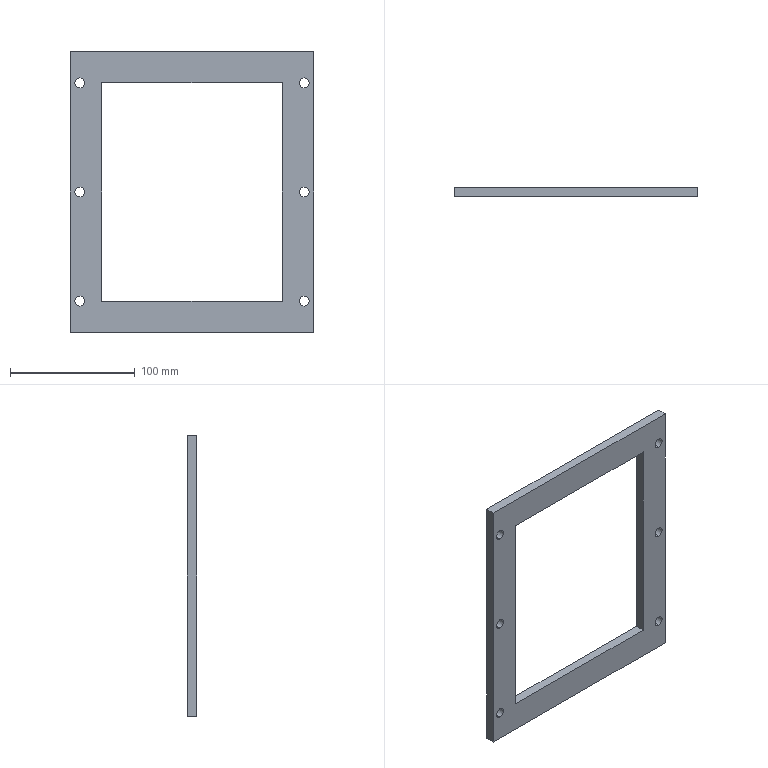Part | STEP file | 2026.6.15-Main Assembly图.sldasm-Part-82 | 1 solid | 22 faces | box 195 x 7.5 x 225 mm | volume 136488 mm3 | cylinder 12 | plane 10 | commonest cylinder face diameters 8 x12
STEP:
#1=CARTESIAN_POINT('',(-1499.224,507.051,4322.667));
#2=VERTEX_POINT('',#1);
#3=CARTESIAN_POINT('',(-1499.224,507.051,4314.667));
#4=VERTEX_POINT('',#3);
#5=CARTESIAN_POINT('',(-1499.224,507.051,4318.667));
#6=DIRECTION('',(0.,-1.,0.));
#7=DIRECTION('',(-1.,0.,0.));
#8=AXIS2_PLACEMENT_3D('',#5,#6,#7);
#9=CIRCLE('',#8,4.);
#10=EDGE_CURVE('',#2,#4,#9,.T.);
#11=ORIENTED_EDGE('',*,*,#10,.F.);
#12=CARTESIAN_POINT('',(-1499.224,499.551,4322.667));
#13=VERTEX_POINT('',#12);
#14=CARTESIAN_POINT('',(-1499.224,507.051,4322.667));
#15=DIRECTION('',(0.,-1.,0.));
#16=VECTOR('',#15,1000.);
#17=LINE('',#14,#16);
#18=EDGE_CURVE('',#2,#13,#17,.T.);
#19=ORIENTED_EDGE('',*,*,#18,.T.);
#20=CARTESIAN_POINT('',(-1499.224,499.551,4314.667));
#21=VERTEX_POINT('',#20);
#22=CARTESIAN_POINT('',(-1499.224,499.551,4318.667));
#23=DIRECTION('',(0.,-1.,0.));
#24=DIRECTION('',(-1.,0.,0.));
#25=AXIS2_PLACEMENT_3D('',#22,#23,#24);
#26=CIRCLE('',#25,4.);
#27=EDGE_CURVE('',#13,#21,#26,.T.);
#28=ORIENTED_EDGE('',*,*,#27,.T.);
#29=CARTESIAN_POINT('',(-1499.224,507.051,4314.667));
#30=DIRECTION('',(0.,-1.,0.));
#31=VECTOR('',#30,1000.);
#32=LINE('',#29,#31);
#33=EDGE_CURVE('',#4,#21,#32,.T.);
#34=ORIENTED_EDGE('',*,*,#33,.F.);
#35=EDGE_LOOP('',(#11,#19,#28,#34));
#36=FACE_OUTER_BOUND('',#35,.T.);
#37=CARTESIAN_POINT('',(-1499.224,507.051,4318.667));
#38=DIRECTION('',(0.,-1.,0.));
#39=DIRECTION('',(0.,0.,-1.));
#40=AXIS2_PLACEMENT_3D('',#37,#38,#39);
#41=CYLINDRICAL_SURFACE('',#40,4.);
#42=ADVANCED_FACE('',(#36),#41,.F.);
#43=CARTESIAN_POINT('',(-1679.224,507.051,4147.667));
#44=VERTEX_POINT('',#43);
#45=CARTESIAN_POINT('',(-1679.224,507.051,4139.667));
#46=VERTEX_POINT('',#45);
#47=CARTESIAN_POINT('',(-1679.224,507.051,4143.667));
#48=DIRECTION('',(0.,-1.,0.));
#49=DIRECTION('',(-1.,0.,0.));
#50=AXIS2_PLACEMENT_3D('',#47,#48,#49);
#51=CIRCLE('',#50,4.);
#52=EDGE_CURVE('',#44,#46,#51,.T.);
#53=ORIENTED_EDGE('',*,*,#52,.F.);
#54=CARTESIAN_POINT('',(-1679.224,499.551,4147.667));
#55=VERTEX_POINT('',#54);
#56=CARTESIAN_POINT('',(-1679.224,507.051,4147.667));
#57=DIRECTION('',(0.,-1.,0.));
#58=VECTOR('',#57,1000.);
#59=LINE('',#56,#58);
#60=EDGE_CURVE('',#44,#55,#59,.T.);
#61=ORIENTED_EDGE('',*,*,#60,.T.);
#62=CARTESIAN_POINT('',(-1679.224,499.551,4139.667));
#63=VERTEX_POINT('',#62);
#64=CARTESIAN_POINT('',(-1679.224,499.551,4143.667));
#65=DIRECTION('',(0.,-1.,0.));
#66=DIRECTION('',(-1.,0.,0.));
#67=AXIS2_PLACEMENT_3D('',#64,#65,#66);
#68=CIRCLE('',#67,4.);
#69=EDGE_CURVE('',#55,#63,#68,.T.);
#70=ORIENTED_EDGE('',*,*,#69,.T.);
#71=CARTESIAN_POINT('',(-1679.224,507.051,4139.667));
#72=DIRECTION('',(0.,-1.,0.));
#73=VECTOR('',#72,1000.);
#74=LINE('',#71,#73);
#75=EDGE_CURVE('',#46,#63,#74,.T.);
#76=ORIENTED_EDGE('',*,*,#75,.F.);
#77=EDGE_LOOP('',(#53,#61,#70,#76));
#78=FACE_OUTER_BOUND('',#77,.T.);
#79=CARTESIAN_POINT('',(-1679.224,507.051,4143.667));
#80=DIRECTION('',(0.,-1.,0.));
#81=DIRECTION('',(0.,0.,-1.));
#82=AXIS2_PLACEMENT_3D('',#79,#80,#81);
#83=CYLINDRICAL_SURFACE('',#82,4.);
#84=ADVANCED_FACE('',(#78),#83,.F.);
#85=CARTESIAN_POINT('',(-1499.224,507.051,4147.667));
#86=VERTEX_POINT('',#85);
#87=CARTESIAN_POINT('',(-1499.224,507.051,4139.667));
#88=VERTEX_POINT('',#87);
#89=CARTESIAN_POINT('',(-1499.224,507.051,4143.667));
#90=DIRECTION('',(0.,-1.,0.));
#91=DIRECTION('',(-1.,0.,0.));
#92=AXIS2_PLACEMENT_3D('',#89,#90,#91);
#93=CIRCLE('',#92,4.);
#94=EDGE_CURVE('',#86,#88,#93,.T.);
#95=ORIENTED_EDGE('',*,*,#94,.F.);
#96=CARTESIAN_POINT('',(-1499.224,499.551,4147.667));
#97=VERTEX_POINT('',#96);
#98=CARTESIAN_POINT('',(-1499.224,507.051,4147.667));
#99=DIRECTION('',(0.,-1.,0.));
#100=VECTOR('',#99,1000.);
#101=LINE('',#98,#100);
#102=EDGE_CURVE('',#86,#97,#101,.T.);
#103=ORIENTED_EDGE('',*,*,#102,.T.);
#104=CARTESIAN_POINT('',(-1499.224,499.551,4139.667));
#105=VERTEX_POINT('',#104);
#106=CARTESIAN_POINT('',(-1499.224,499.551,4143.667));
#107=DIRECTION('',(0.,-1.,0.));
#108=DIRECTION('',(-1.,0.,0.));
#109=AXIS2_PLACEMENT_3D('',#106,#107,#108);
#110=CIRCLE('',#109,4.);
#111=EDGE_CURVE('',#97,#105,#110,.T.);
#112=ORIENTED_EDGE('',*,*,#111,.T.);
#113=CARTESIAN_POINT('',(-1499.224,507.051,4139.667));
#114=DIRECTION('',(0.,-1.,0.));
#115=VECTOR('',#114,1000.);
#116=LINE('',#113,#115);
#117=EDGE_CURVE('',#88,#105,#116,.T.);
#118=ORIENTED_EDGE('',*,*,#117,.F.);
#119=EDGE_LOOP('',(#95,#103,#112,#118));
#120=FACE_OUTER_BOUND('',#119,.T.);
#121=CARTESIAN_POINT('',(-1499.224,507.051,4143.667));
#122=DIRECTION('',(0.,-1.,0.));
#123=DIRECTION('',(0.,0.,-1.));
#124=AXIS2_PLACEMENT_3D('',#121,#122,#123);
#125=CYLINDRICAL_SURFACE('',#124,4.);
#126=ADVANCED_FACE('',(#120),#125,.F.);
#127=CARTESIAN_POINT('',(-1679.224,507.051,4235.167));
#128=VERTEX_POINT('',#127);
#129=CARTESIAN_POINT('',(-1679.224,507.051,4227.167));
#130=VERTEX_POINT('',#129);
#131=CARTESIAN_POINT('',(-1679.224,507.051,4231.167));
#132=DIRECTION('',(0.,-1.,0.));
#133=DIRECTION('',(-1.,0.,0.));
#134=AXIS2_PLACEMENT_3D('',#131,#132,#133);
#135=CIRCLE('',#134,4.);
#136=EDGE_CURVE('',#128,#130,#135,.T.);
#137=ORIENTED_EDGE('',*,*,#136,.F.);
#138=CARTESIAN_POINT('',(-1679.224,499.551,4235.167));
#139=VERTEX_POINT('',#138);
#140=CARTESIAN_POINT('',(-1679.224,507.051,4235.167));
#141=DIRECTION('',(0.,-1.,0.));
#142=VECTOR('',#141,1000.);
#143=LINE('',#140,#142);
#144=EDGE_CURVE('',#128,#139,#143,.T.);
#145=ORIENTED_EDGE('',*,*,#144,.T.);
#146=CARTESIAN_POINT('',(-1679.224,499.551,4227.167));
#147=VERTEX_POINT('',#146);
#148=CARTESIAN_POINT('',(-1679.224,499.551,4231.167));
#149=DIRECTION('',(0.,-1.,0.));
#150=DIRECTION('',(-1.,0.,0.));
#151=AXIS2_PLACEMENT_3D('',#148,#149,#150);
#152=CIRCLE('',#151,4.);
#153=EDGE_CURVE('',#139,#147,#152,.T.);
#154=ORIENTED_EDGE('',*,*,#153,.T.);
#155=CARTESIAN_POINT('',(-1679.224,507.051,4227.167));
#156=DIRECTION('',(0.,-1.,0.));
#157=VECTOR('',#156,1000.);
#158=LINE('',#155,#157);
#159=EDGE_CURVE('',#130,#147,#158,.T.);
#160=ORIENTED_EDGE('',*,*,#159,.F.);
#161=EDGE_LOOP('',(#137,#145,#154,#160));
#162=FACE_OUTER_BOUND('',#161,.T.);
#163=CARTESIAN_POINT('',(-1679.224,507.051,4231.167));
#164=DIRECTION('',(0.,-1.,0.));
#165=DIRECTION('',(0.,0.,-1.));
#166=AXIS2_PLACEMENT_3D('',#163,#164,#165);
#167=CYLINDRICAL_SURFACE('',#166,4.);
#168=ADVANCED_FACE('',(#162),#167,.F.);
#169=CARTESIAN_POINT('',(-1499.224,507.051,4235.167));
#170=VERTEX_POINT('',#169);
#171=CARTESIAN_POINT('',(-1499.224,507.051,4227.167));
#172=VERTEX_POINT('',#171);
#173=CARTESIAN_POINT('',(-1499.224,507.051,4231.167));
#174=DIRECTION('',(0.,-1.,0.));
#175=DIRECTION('',(-1.,0.,0.));
#176=AXIS2_PLACEMENT_3D('',#173,#174,#175);
#177=CIRCLE('',#176,4.);
#178=EDGE_CURVE('',#170,#172,#177,.T.);
#179=ORIENTED_EDGE('',*,*,#178,.F.);
#180=CARTESIAN_POINT('',(-1499.224,499.551,4235.167));
#181=VERTEX_POINT('',#180);
#182=CARTESIAN_POINT('',(-1499.224,507.051,4235.167));
#183=DIRECTION('',(0.,-1.,0.));
#184=VECTOR('',#183,1000.);
#185=LINE('',#182,#184);
#186=EDGE_CURVE('',#170,#181,#185,.T.);
#187=ORIENTED_EDGE('',*,*,#186,.T.);
#188=CARTESIAN_POINT('',(-1499.224,499.551,4227.167));
#189=VERTEX_POINT('',#188);
#190=CARTESIAN_POINT('',(-1499.224,499.551,4231.167));
#191=DIRECTION('',(0.,-1.,0.));
#192=DIRECTION('',(-1.,0.,0.));
#193=AXIS2_PLACEMENT_3D('',#190,#191,#192);
#194=CIRCLE('',#193,4.);
#195=EDGE_CURVE('',#181,#189,#194,.T.);
#196=ORIENTED_EDGE('',*,*,#195,.T.);
#197=CARTESIAN_POINT('',(-1499.224,507.051,4227.167));
#198=DIRECTION('',(0.,-1.,0.));
#199=VECTOR('',#198,1000.);
#200=LINE('',#197,#199);
#201=EDGE_CURVE('',#172,#189,#200,.T.);
#202=ORIENTED_EDGE('',*,*,#201,.F.);
#203=EDGE_LOOP('',(#179,#187,#196,#202));
#204=FACE_OUTER_BOUND('',#203,.T.);
#205=CARTESIAN_POINT('',(-1499.224,507.051,4231.167));
#206=DIRECTION('',(0.,-1.,0.));
#207=DIRECTION('',(0.,0.,-1.));
#208=AXIS2_PLACEMENT_3D('',#205,#206,#207);
#209=CYLINDRICAL_SURFACE('',#208,4.);
#210=ADVANCED_FACE('',(#204),#209,.F.);
#211=CARTESIAN_POINT('',(-1679.224,507.051,4322.667));
#212=VERTEX_POINT('',#211);
#213=CARTESIAN_POINT('',(-1679.224,507.051,4314.667));
#214=VERTEX_POINT('',#213);
#215=CARTESIAN_POINT('',(-1679.224,507.051,4318.667));
#216=DIRECTION('',(0.,-1.,0.));
#217=DIRECTION('',(-1.,0.,0.));
#218=AXIS2_PLACEMENT_3D('',#215,#216,#217);
#219=CIRCLE('',#218,4.);
#220=EDGE_CURVE('',#212,#214,#219,.T.);
#221=ORIENTED_EDGE('',*,*,#220,.F.);
#222=CARTESIAN_POINT('',(-1679.224,499.551,4322.667));
#223=VERTEX_POINT('',#222);
#224=CARTESIAN_POINT('',(-1679.224,507.051,4322.667));
#225=DIRECTION('',(0.,-1.,0.));
#226=VECTOR('',#225,1000.);
#227=LINE('',#224,#226);
#228=EDGE_CURVE('',#212,#223,#227,.T.);
#229=ORIENTED_EDGE('',*,*,#228,.T.);
#230=CARTESIAN_POINT('',(-1679.224,499.551,4314.667));
#231=VERTEX_POINT('',#230);
#232=CARTESIAN_POINT('',(-1679.224,499.551,4318.667));
#233=DIRECTION('',(0.,-1.,0.));
#234=DIRECTION('',(-1.,0.,0.));
#235=AXIS2_PLACEMENT_3D('',#232,#233,#234);
#236=CIRCLE('',#235,4.);
#237=EDGE_CURVE('',#223,#231,#236,.T.);
#238=ORIENTED_EDGE('',*,*,#237,.T.);
#239=CARTESIAN_POINT('',(-1679.224,507.051,4314.667));
#240=DIRECTION('',(0.,-1.,0.));
#241=VECTOR('',#240,1000.);
#242=LINE('',#239,#241);
#243=EDGE_CURVE('',#214,#231,#242,.T.);
#244=ORIENTED_EDGE('',*,*,#243,.F.);
#245=EDGE_LOOP('',(#221,#229,#238,#244));
#246=FACE_OUTER_BOUND('',#245,.T.);
#247=CARTESIAN_POINT('',(-1679.224,507.051,4318.667));
#248=DIRECTION('',(0.,-1.,0.));
#249=DIRECTION('',(0.,0.,-1.));
#250=AXIS2_PLACEMENT_3D('',#247,#248,#249);
#251=CYLINDRICAL_SURFACE('',#250,4.);
#252=ADVANCED_FACE('',(#246),#251,.F.);
#253=CARTESIAN_POINT('',(-1661.724,499.551,4143.667));
#254=VERTEX_POINT('',#253);
#255=CARTESIAN_POINT('',(-1516.724,499.551,4143.667));
#256=VERTEX_POINT('',#255);
#257=CARTESIAN_POINT('',(-1661.724,499.551,4143.667));
#258=DIRECTION('',(1.,0.,0.));
#259=VECTOR('',#258,1000.);
#260=LINE('',#257,#259);
#261=EDGE_CURVE('',#254,#256,#260,.T.);
#262=ORIENTED_EDGE('',*,*,#261,.T.);
#263=CARTESIAN_POINT('',(-1516.724,507.051,4143.667));
#264=VERTEX_POINT('',#263);
#265=CARTESIAN_POINT('',(-1516.724,507.051,4143.667));
#266=DIRECTION('',(0.,-1.,0.));
#267=VECTOR('',#266,1000.);
#268=LINE('',#265,#267);
#269=EDGE_CURVE('',#264,#256,#268,.T.);
#270=ORIENTED_EDGE('',*,*,#269,.F.);
#271=CARTESIAN_POINT('',(-1661.724,507.051,4143.667));
#272=VERTEX_POINT('',#271);
#273=CARTESIAN_POINT('',(-1661.724,507.051,4143.667));
#274=DIRECTION('',(1.,0.,0.));
#275=VECTOR('',#274,1000.);
#276=LINE('',#273,#275);
#277=EDGE_CURVE('',#272,#264,#276,.T.);
#278=ORIENTED_EDGE('',*,*,#277,.F.);
#279=CARTESIAN_POINT('',(-1661.724,507.051,4143.667));
#280=DIRECTION('',(0.,-1.,0.));
#281=VECTOR('',#280,1000.);
#282=LINE('',#279,#281);
#283=EDGE_CURVE('',#272,#254,#282,.T.);
#284=ORIENTED_EDGE('',*,*,#283,.T.);
#285=EDGE_LOOP('',(#262,#270,#278,#284));
#286=FACE_OUTER_BOUND('',#285,.T.);
#287=CARTESIAN_POINT('',(-1661.724,507.051,4143.667));
#288=DIRECTION('',(0.,0.,-1.));
#289=DIRECTION('',(-1.,0.,0.));
#290=AXIS2_PLACEMENT_3D('',#287,#288,#289);
#291=PLANE('',#290);
#292=ADVANCED_FACE('',(#286),#291,.F.);
#293=CARTESIAN_POINT('',(-1516.724,499.551,4318.667));
#294=VERTEX_POINT('',#293);
#295=CARTESIAN_POINT('',(-1516.724,499.551,4143.667));
#296=DIRECTION('',(0.,0.,1.));
#297=VECTOR('',#296,1000.);
#298=LINE('',#295,#297);
#299=EDGE_CURVE('',#256,#294,#298,.T.);
#300=ORIENTED_EDGE('',*,*,#299,.T.);
#301=CARTESIAN_POINT('',(-1516.724,507.051,4318.667));
#302=VERTEX_POINT('',#301);
#303=CARTESIAN_POINT('',(-1516.724,507.051,4318.667));
#304=DIRECTION('',(0.,-1.,0.));
#305=VECTOR('',#304,1000.);
#306=LINE('',#303,#305);
#307=EDGE_CURVE('',#302,#294,#306,.T.);
#308=ORIENTED_EDGE('',*,*,#307,.F.);
#309=CARTESIAN_POINT('',(-1516.724,507.051,4143.667));
#310=DIRECTION('',(0.,0.,1.));
#311=VECTOR('',#310,1000.);
#312=LINE('',#309,#311);
#313=EDGE_CURVE('',#264,#302,#312,.T.);
#314=ORIENTED_EDGE('',*,*,#313,.F.);
#315=ORIENTED_EDGE('',*,*,#269,.T.);
#316=EDGE_LOOP('',(#300,#308,#314,#315));
#317=FACE_OUTER_BOUND('',#316,.T.);
#318=CARTESIAN_POINT('',(-1516.724,507.051,4143.667));
#319=DIRECTION('',(1.,0.,0.));
#320=DIRECTION('',(0.,0.,-1.));
#321=AXIS2_PLACEMENT_3D('',#318,#319,#320);
#322=PLANE('',#321);
#323=ADVANCED_FACE('',(#317),#322,.F.);
#324=CARTESIAN_POINT('',(-1661.724,499.551,4318.667));
#325=VERTEX_POINT('',#324);
#326=CARTESIAN_POINT('',(-1516.724,499.551,4318.667));
#327=DIRECTION('',(-1.,0.,0.));
#328=VECTOR('',#327,1000.);
#329=LINE('',#326,#328);
#330=EDGE_CURVE('',#294,#325,#329,.T.);
#331=ORIENTED_EDGE('',*,*,#330,.T.);
#332=CARTESIAN_POINT('',(-1661.724,507.051,4318.667));
#333=VERTEX_POINT('',#332);
#334=CARTESIAN_POINT('',(-1661.724,507.051,4318.667));
#335=DIRECTION('',(0.,-1.,0.));
#336=VECTOR('',#335,1000.);
#337=LINE('',#334,#336);
#338=EDGE_CURVE('',#333,#325,#337,.T.);
#339=ORIENTED_EDGE('',*,*,#338,.F.);
#340=CARTESIAN_POINT('',(-1516.724,507.051,4318.667));
#341=DIRECTION('',(-1.,0.,0.));
#342=VECTOR('',#341,1000.);
#343=LINE('',#340,#342);
#344=EDGE_CURVE('',#302,#333,#343,.T.);
#345=ORIENTED_EDGE('',*,*,#344,.F.);
#346=ORIENTED_EDGE('',*,*,#307,.T.);
#347=EDGE_LOOP('',(#331,#339,#345,#346));
#348=FACE_OUTER_BOUND('',#347,.T.);
#349=CARTESIAN_POINT('',(-1516.724,507.051,4318.667));
#350=DIRECTION('',(0.,0.,1.));
#351=DIRECTION('',(1.,0.,0.));
#352=AXIS2_PLACEMENT_3D('',#349,#350,#351);
#353=PLANE('',#352);
#354=ADVANCED_FACE('',(#348),#353,.F.);
#355=CARTESIAN_POINT('',(-1491.724,499.551,4118.667));
#356=VERTEX_POINT('',#355);
#357=CARTESIAN_POINT('',(-1686.724,499.551,4118.667));
#358=VERTEX_POINT('',#357);
#359=CARTESIAN_POINT('',(-1491.724,499.551,4118.667));
#360=DIRECTION('',(-1.,0.,0.));
#361=VECTOR('',#360,1000.);
#362=LINE('',#359,#361);
#363=EDGE_CURVE('',#356,#358,#362,.T.);
#364=ORIENTED_EDGE('',*,*,#363,.T.);
#365=CARTESIAN_POINT('',(-1686.724,507.051,4118.667));
#366=VERTEX_POINT('',#365);
#367=CARTESIAN_POINT('',(-1686.724,507.051,4118.667));
#368=DIRECTION('',(0.,-1.,0.));
#369=VECTOR('',#368,1000.);
#370=LINE('',#367,#369);
#371=EDGE_CURVE('',#366,#358,#370,.T.);
#372=ORIENTED_EDGE('',*,*,#371,.F.);
#373=CARTESIAN_POINT('',(-1491.724,507.051,4118.667));
#374=VERTEX_POINT('',#373);
#375=CARTESIAN_POINT('',(-1491.724,507.051,4118.667));
#376=DIRECTION('',(-1.,0.,0.));
#377=VECTOR('',#376,1000.);
#378=LINE('',#375,#377);
#379=EDGE_CURVE('',#374,#366,#378,.T.);
#380=ORIENTED_EDGE('',*,*,#379,.F.);
#381=CARTESIAN_POINT('',(-1491.724,507.051,4118.667));
#382=DIRECTION('',(0.,-1.,0.));
#383=VECTOR('',#382,1000.);
#384=LINE('',#381,#383);
#385=EDGE_CURVE('',#374,#356,#384,.T.);
#386=ORIENTED_EDGE('',*,*,#385,.T.);
#387=EDGE_LOOP('',(#364,#372,#380,#386));
#388=FACE_OUTER_BOUND('',#387,.T.);
#389=CARTESIAN_POINT('',(-1491.724,507.051,4118.667));
#390=DIRECTION('',(0.,0.,1.));
#391=DIRECTION('',(1.,0.,0.));
#392=AXIS2_PLACEMENT_3D('',#389,#390,#391);
#393=PLANE('',#392);
#394=ADVANCED_FACE('',(#388),#393,.F.);
#395=CARTESIAN_POINT('',(-1686.724,499.551,4343.667));
#396=VERTEX_POINT('',#395);
#397=CARTESIAN_POINT('',(-1686.724,499.551,4118.667));
#398=DIRECTION('',(0.,0.,1.));
#399=VECTOR('',#398,1000.);
#400=LINE('',#397,#399);
#401=EDGE_CURVE('',#358,#396,#400,.T.);
#402=ORIENTED_EDGE('',*,*,#401,.T.);
#403=CARTESIAN_POINT('',(-1686.724,507.051,4343.667));
#404=VERTEX_POINT('',#403);
#405=CARTESIAN_POINT('',(-1686.724,507.051,4343.667));
#406=DIRECTION('',(0.,-1.,0.));
#407=VECTOR('',#406,1000.);
#408=LINE('',#405,#407);
#409=EDGE_CURVE('',#404,#396,#408,.T.);
#410=ORIENTED_EDGE('',*,*,#409,.F.);
#411=CARTESIAN_POINT('',(-1686.724,507.051,4118.667));
#412=DIRECTION('',(0.,0.,1.));
#413=VECTOR('',#412,1000.);
#414=LINE('',#411,#413);
#415=EDGE_CURVE('',#366,#404,#414,.T.);
#416=ORIENTED_EDGE('',*,*,#415,.F.);
#417=ORIENTED_EDGE('',*,*,#371,.T.);
#418=EDGE_LOOP('',(#402,#410,#416,#417));
#419=FACE_OUTER_BOUND('',#418,.T.);
#420=CARTESIAN_POINT('',(-1686.724,507.051,4118.667));
#421=DIRECTION('',(1.,0.,0.));
#422=DIRECTION('',(0.,0.,-1.));
#423=AXIS2_PLACEMENT_3D('',#420,#421,#422);
#424=PLANE('',#423);
#425=ADVANCED_FACE('',(#419),#424,.F.);
#426=CARTESIAN_POINT('',(-1491.724,499.551,4343.667));
#427=VERTEX_POINT('',#426);
#428=CARTESIAN_POINT('',(-1686.724,499.551,4343.667));
#429=DIRECTION('',(1.,0.,0.));
#430=VECTOR('',#429,1000.);
#431=LINE('',#428,#430);
#432=EDGE_CURVE('',#396,#427,#431,.T.);
#433=ORIENTED_EDGE('',*,*,#432,.T.);
#434=CARTESIAN_POINT('',(-1491.724,507.051,4343.667));
#435=VERTEX_POINT('',#434);
#436=CARTESIAN_POINT('',(-1491.724,507.051,4343.667));
#437=DIRECTION('',(0.,-1.,0.));
#438=VECTOR('',#437,1000.);
#439=LINE('',#436,#438);
#440=EDGE_CURVE('',#435,#427,#439,.T.);
#441=ORIENTED_EDGE('',*,*,#440,.F.);
#442=CARTESIAN_POINT('',(-1686.724,507.051,4343.667));
#443=DIRECTION('',(1.,0.,0.));
#444=VECTOR('',#443,1000.);
#445=LINE('',#442,#444);
#446=EDGE_CURVE('',#404,#435,#445,.T.);
#447=ORIENTED_EDGE('',*,*,#446,.F.);
#448=ORIENTED_EDGE('',*,*,#409,.T.);
#449=EDGE_LOOP('',(#433,#441,#447,#448));
#450=FACE_OUTER_BOUND('',#449,.T.);
#451=CARTESIAN_POINT('',(-1686.724,507.051,4343.667));
#452=DIRECTION('',(0.,0.,-1.));
#453=DIRECTION('',(-1.,0.,0.));
#454=AXIS2_PLACEMENT_3D('',#451,#452,#453);
#455=PLANE('',#454);
#456=ADVANCED_FACE('',(#450),#455,.F.);
#457=ORIENTED_EDGE('',*,*,#228,.F.);
#458=CARTESIAN_POINT('',(-1679.224,507.051,4318.667));
#459=DIRECTION('',(0.,-1.,0.));
#460=DIRECTION('',(-1.,0.,0.));
#461=AXIS2_PLACEMENT_3D('',#458,#459,#460);
#462=CIRCLE('',#461,4.);
#463=EDGE_CURVE('',#214,#212,#462,.T.);
#464=ORIENTED_EDGE('',*,*,#463,.F.);
#465=ORIENTED_EDGE('',*,*,#243,.T.);
#466=CARTESIAN_POINT('',(-1679.224,499.551,4318.667));
#467=DIRECTION('',(0.,-1.,0.));
#468=DIRECTION('',(-1.,0.,0.));
#469=AXIS2_PLACEMENT_3D('',#466,#467,#468);
#470=CIRCLE('',#469,4.);
#471=EDGE_CURVE('',#231,#223,#470,.T.);
#472=ORIENTED_EDGE('',*,*,#471,.T.);
#473=EDGE_LOOP('',(#457,#464,#465,#472));
#474=FACE_OUTER_BOUND('',#473,.T.);
#475=CARTESIAN_POINT('',(-1679.224,507.051,4318.667));
#476=DIRECTION('',(0.,-1.,0.));
#477=DIRECTION('',(0.,0.,-1.));
#478=AXIS2_PLACEMENT_3D('',#475,#476,#477);
#479=CYLINDRICAL_SURFACE('',#478,4.);
#480=ADVANCED_FACE('',(#474),#479,.F.);
#481=ORIENTED_EDGE('',*,*,#186,.F.);
#482=CARTESIAN_POINT('',(-1499.224,507.051,4231.167));
#483=DIRECTION('',(0.,-1.,0.));
#484=DIRECTION('',(-1.,0.,0.));
#485=AXIS2_PLACEMENT_3D('',#482,#483,#484);
#486=CIRCLE('',#485,4.);
#487=EDGE_CURVE('',#172,#170,#486,.T.);
#488=ORIENTED_EDGE('',*,*,#487,.F.);
#489=ORIENTED_EDGE('',*,*,#201,.T.);
#490=CARTESIAN_POINT('',(-1499.224,499.551,4231.167));
#491=DIRECTION('',(0.,-1.,0.));
#492=DIRECTION('',(-1.,0.,0.));
#493=AXIS2_PLACEMENT_3D('',#490,#491,#492);
#494=CIRCLE('',#493,4.);
#495=EDGE_CURVE('',#189,#181,#494,.T.);
#496=ORIENTED_EDGE('',*,*,#495,.T.);
#497=EDGE_LOOP('',(#481,#488,#489,#496));
#498=FACE_OUTER_BOUND('',#497,.T.);
#499=CARTESIAN_POINT('',(-1499.224,507.051,4231.167));
#500=DIRECTION('',(0.,-1.,0.));
#501=DIRECTION('',(0.,0.,-1.));
#502=AXIS2_PLACEMENT_3D('',#499,#500,#501);
#503=CYLINDRICAL_SURFACE('',#502,4.);
#504=ADVANCED_FACE('',(#498),#503,.F.);
#505=ORIENTED_EDGE('',*,*,#144,.F.);
#506=CARTESIAN_POINT('',(-1679.224,507.051,4231.167));
#507=DIRECTION('',(0.,-1.,0.));
#508=DIRECTION('',(-1.,0.,0.));
#509=AXIS2_PLACEMENT_3D('',#506,#507,#508);
#510=CIRCLE('',#509,4.);
#511=EDGE_CURVE('',#130,#128,#510,.T.);
#512=ORIENTED_EDGE('',*,*,#511,.F.);
#513=ORIENTED_EDGE('',*,*,#159,.T.);
#514=CARTESIAN_POINT('',(-1679.224,499.551,4231.167));
#515=DIRECTION('',(0.,-1.,0.));
#516=DIRECTION('',(-1.,0.,0.));
#517=AXIS2_PLACEMENT_3D('',#514,#515,#516);
#518=CIRCLE('',#517,4.);
#519=EDGE_CURVE('',#147,#139,#518,.T.);
#520=ORIENTED_EDGE('',*,*,#519,.T.);
#521=EDGE_LOOP('',(#505,#512,#513,#520));
#522=FACE_OUTER_BOUND('',#521,.T.);
#523=CARTESIAN_POINT('',(-1679.224,507.051,4231.167));
#524=DIRECTION('',(0.,-1.,0.));
#525=DIRECTION('',(0.,0.,-1.));
#526=AXIS2_PLACEMENT_3D('',#523,#524,#525);
#527=CYLINDRICAL_SURFACE('',#526,4.);
#528=ADVANCED_FACE('',(#522),#527,.F.);
#529=ORIENTED_EDGE('',*,*,#102,.F.);
#530=CARTESIAN_POINT('',(-1499.224,507.051,4143.667));
#531=DIRECTION('',(0.,-1.,0.));
#532=DIRECTION('',(-1.,0.,0.));
#533=AXIS2_PLACEMENT_3D('',#530,#531,#532);
#534=CIRCLE('',#533,4.);
#535=EDGE_CURVE('',#88,#86,#534,.T.);
#536=ORIENTED_EDGE('',*,*,#535,.F.);
#537=ORIENTED_EDGE('',*,*,#117,.T.);
#538=CARTESIAN_POINT('',(-1499.224,499.551,4143.667));
#539=DIRECTION('',(0.,-1.,0.));
#540=DIRECTION('',(-1.,0.,0.));
#541=AXIS2_PLACEMENT_3D('',#538,#539,#540);
#542=CIRCLE('',#541,4.);
#543=EDGE_CURVE('',#105,#97,#542,.T.);
#544=ORIENTED_EDGE('',*,*,#543,.T.);
#545=EDGE_LOOP('',(#529,#536,#537,#544));
#546=FACE_OUTER_BOUND('',#545,.T.);
#547=CARTESIAN_POINT('',(-1499.224,507.051,4143.667));
#548=DIRECTION('',(0.,-1.,0.));
#549=DIRECTION('',(0.,0.,-1.));
#550=AXIS2_PLACEMENT_3D('',#547,#548,#549);
#551=CYLINDRICAL_SURFACE('',#550,4.);
#552=ADVANCED_FACE('',(#546),#551,.F.);
#553=CARTESIAN_POINT('',(-1661.724,499.551,4318.667));
#554=DIRECTION('',(0.,0.,-1.));
#555=VECTOR('',#554,1000.);
#556=LINE('',#553,#555);
#557=EDGE_CURVE('',#325,#254,#556,.T.);
#558=ORIENTED_EDGE('',*,*,#557,.T.);
#559=ORIENTED_EDGE('',*,*,#283,.F.);
#560=CARTESIAN_POINT('',(-1661.724,507.051,4318.667));
#561=DIRECTION('',(0.,0.,-1.));
#562=VECTOR('',#561,1000.);
#563=LINE('',#560,#562);
#564=EDGE_CURVE('',#333,#272,#563,.T.);
#565=ORIENTED_EDGE('',*,*,#564,.F.);
#566=ORIENTED_EDGE('',*,*,#338,.T.);
#567=EDGE_LOOP('',(#558,#559,#565,#566));
#568=FACE_OUTER_BOUND('',#567,.T.);
#569=CARTESIAN_POINT('',(-1661.724,507.051,4318.667));
#570=DIRECTION('',(-1.,0.,0.));
#571=DIRECTION('',(0.,0.,1.));
#572=AXIS2_PLACEMENT_3D('',#569,#570,#571);
#573=PLANE('',#572);
#574=ADVANCED_FACE('',(#568),#573,.F.);
#575=ORIENTED_EDGE('',*,*,#60,.F.);
#576=CARTESIAN_POINT('',(-1679.224,507.051,4143.667));
#577=DIRECTION('',(0.,-1.,0.));
#578=DIRECTION('',(-1.,0.,0.));
#579=AXIS2_PLACEMENT_3D('',#576,#577,#578);
#580=CIRCLE('',#579,4.);
#581=EDGE_CURVE('',#46,#44,#580,.T.);
#582=ORIENTED_EDGE('',*,*,#581,.F.);
#583=ORIENTED_EDGE('',*,*,#75,.T.);
#584=CARTESIAN_POINT('',(-1679.224,499.551,4143.667));
#585=DIRECTION('',(0.,-1.,0.));
#586=DIRECTION('',(-1.,0.,0.));
#587=AXIS2_PLACEMENT_3D('',#584,#585,#586);
#588=CIRCLE('',#587,4.);
#589=EDGE_CURVE('',#63,#55,#588,.T.);
#590=ORIENTED_EDGE('',*,*,#589,.T.);
#591=EDGE_LOOP('',(#575,#582,#583,#590));
#592=FACE_OUTER_BOUND('',#591,.T.);
#593=CARTESIAN_POINT('',(-1679.224,507.051,4143.667));
#594=DIRECTION('',(0.,-1.,0.));
#595=DIRECTION('',(0.,0.,-1.));
#596=AXIS2_PLACEMENT_3D('',#593,#594,#595);
#597=CYLINDRICAL_SURFACE('',#596,4.);
#598=ADVANCED_FACE('',(#592),#597,.F.);
#599=CARTESIAN_POINT('',(-1491.724,499.551,4343.667));
#600=DIRECTION('',(0.,0.,-1.));
#601=VECTOR('',#600,1000.);
#602=LINE('',#599,#601);
#603=EDGE_CURVE('',#427,#356,#602,.T.);
#604=ORIENTED_EDGE('',*,*,#603,.T.);
#605=ORIENTED_EDGE('',*,*,#385,.F.);
#606=CARTESIAN_POINT('',(-1491.724,507.051,4343.667));
#607=DIRECTION('',(0.,0.,-1.));
#608=VECTOR('',#607,1000.);
#609=LINE('',#606,#608);
#610=EDGE_CURVE('',#435,#374,#609,.T.);
#611=ORIENTED_EDGE('',*,*,#610,.F.);
#612=ORIENTED_EDGE('',*,*,#440,.T.);
#613=EDGE_LOOP('',(#604,#605,#611,#612));
#614=FACE_OUTER_BOUND('',#613,.T.);
#615=CARTESIAN_POINT('',(-1491.724,507.051,4343.667));
#616=DIRECTION('',(-1.,0.,0.));
#617=DIRECTION('',(0.,0.,1.));
#618=AXIS2_PLACEMENT_3D('',#615,#616,#617);
#619=PLANE('',#618);
#620=ADVANCED_FACE('',(#614),#619,.F.);
#621=ORIENTED_EDGE('',*,*,#18,.F.);
#622=CARTESIAN_POINT('',(-1499.224,507.051,4318.667));
#623=DIRECTION('',(0.,-1.,0.));
#624=DIRECTION('',(-1.,0.,0.));
#625=AXIS2_PLACEMENT_3D('',#622,#623,#624);
#626=CIRCLE('',#625,4.);
#627=EDGE_CURVE('',#4,#2,#626,.T.);
#628=ORIENTED_EDGE('',*,*,#627,.F.);
#629=ORIENTED_EDGE('',*,*,#33,.T.);
#630=CARTESIAN_POINT('',(-1499.224,499.551,4318.667));
#631=DIRECTION('',(0.,-1.,0.));
#632=DIRECTION('',(-1.,0.,0.));
#633=AXIS2_PLACEMENT_3D('',#630,#631,#632);
#634=CIRCLE('',#633,4.);
#635=EDGE_CURVE('',#21,#13,#634,.T.);
#636=ORIENTED_EDGE('',*,*,#635,.T.);
#637=EDGE_LOOP('',(#621,#628,#629,#636));
#638=FACE_OUTER_BOUND('',#637,.T.);
#639=CARTESIAN_POINT('',(-1499.224,507.051,4318.667));
#640=DIRECTION('',(0.,-1.,0.));
#641=DIRECTION('',(0.,0.,-1.));
#642=AXIS2_PLACEMENT_3D('',#639,#640,#641);
#643=CYLINDRICAL_SURFACE('',#642,4.);
#644=ADVANCED_FACE('',(#638),#643,.F.);
#645=ORIENTED_EDGE('',*,*,#379,.T.);
#646=ORIENTED_EDGE('',*,*,#415,.T.);
#647=ORIENTED_EDGE('',*,*,#446,.T.);
#648=ORIENTED_EDGE('',*,*,#610,.T.);
#649=EDGE_LOOP('',(#645,#646,#647,#648));
#650=FACE_OUTER_BOUND('',#649,.T.);
#651=ORIENTED_EDGE('',*,*,#581,.T.);
#652=ORIENTED_EDGE('',*,*,#52,.T.);
#653=EDGE_LOOP('',(#651,#652));
#654=FACE_BOUND('',#653,.T.);
#655=ORIENTED_EDGE('',*,*,#277,.T.);
#656=ORIENTED_EDGE('',*,*,#313,.T.);
#657=ORIENTED_EDGE('',*,*,#344,.T.);
#658=ORIENTED_EDGE('',*,*,#564,.T.);
#659=EDGE_LOOP('',(#655,#656,#657,#658));
#660=FACE_BOUND('',#659,.T.);
#661=ORIENTED_EDGE('',*,*,#535,.T.);
#662=ORIENTED_EDGE('',*,*,#94,.T.);
#663=EDGE_LOOP('',(#661,#662));
#664=FACE_BOUND('',#663,.T.);
#665=ORIENTED_EDGE('',*,*,#511,.T.);
#666=ORIENTED_EDGE('',*,*,#136,.T.);
#667=EDGE_LOOP('',(#665,#666));
#668=FACE_BOUND('',#667,.T.);
#669=ORIENTED_EDGE('',*,*,#487,.T.);
#670=ORIENTED_EDGE('',*,*,#178,.T.);
#671=EDGE_LOOP('',(#669,#670));
#672=FACE_BOUND('',#671,.T.);
#673=ORIENTED_EDGE('',*,*,#463,.T.);
#674=ORIENTED_EDGE('',*,*,#220,.T.);
#675=EDGE_LOOP('',(#673,#674));
#676=FACE_BOUND('',#675,.T.);
#677=ORIENTED_EDGE('',*,*,#627,.T.);
#678=ORIENTED_EDGE('',*,*,#10,.T.);
#679=EDGE_LOOP('',(#677,#678));
#680=FACE_BOUND('',#679,.T.);
#681=CARTESIAN_POINT('',(-1679.224,507.051,4143.667));
#682=DIRECTION('',(0.,-1.,0.));
#683=DIRECTION('',(0.,0.,-1.));
#684=AXIS2_PLACEMENT_3D('',#681,#682,#683);
#685=PLANE('',#684);
#686=ADVANCED_FACE('',(#650,#654,#660,#664,#668,#672,#676,#680),#685,.F.);
#687=ORIENTED_EDGE('',*,*,#363,.F.);
#688=ORIENTED_EDGE('',*,*,#603,.F.);
#689=ORIENTED_EDGE('',*,*,#432,.F.);
#690=ORIENTED_EDGE('',*,*,#401,.F.);
#691=EDGE_LOOP('',(#687,#688,#689,#690));
#692=FACE_OUTER_BOUND('',#691,.T.);
#693=ORIENTED_EDGE('',*,*,#589,.F.);
#694=ORIENTED_EDGE('',*,*,#69,.F.);
#695=EDGE_LOOP('',(#693,#694));
#696=FACE_BOUND('',#695,.T.);
#697=ORIENTED_EDGE('',*,*,#261,.F.);
#698=ORIENTED_EDGE('',*,*,#557,.F.);
#699=ORIENTED_EDGE('',*,*,#330,.F.);
#700=ORIENTED_EDGE('',*,*,#299,.F.);
#701=EDGE_LOOP('',(#697,#698,#699,#700));
#702=FACE_BOUND('',#701,.T.);
#703=ORIENTED_EDGE('',*,*,#543,.F.);
#704=ORIENTED_EDGE('',*,*,#111,.F.);
#705=EDGE_LOOP('',(#703,#704));
#706=FACE_BOUND('',#705,.T.);
#707=ORIENTED_EDGE('',*,*,#519,.F.);
#708=ORIENTED_EDGE('',*,*,#153,.F.);
#709=EDGE_LOOP('',(#707,#708));
#710=FACE_BOUND('',#709,.T.);
#711=ORIENTED_EDGE('',*,*,#495,.F.);
#712=ORIENTED_EDGE('',*,*,#195,.F.);
#713=EDGE_LOOP('',(#711,#712));
#714=FACE_BOUND('',#713,.T.);
#715=ORIENTED_EDGE('',*,*,#471,.F.);
#716=ORIENTED_EDGE('',*,*,#237,.F.);
#717=EDGE_LOOP('',(#715,#716));
#718=FACE_BOUND('',#717,.T.);
#719=ORIENTED_EDGE('',*,*,#635,.F.);
#720=ORIENTED_EDGE('',*,*,#27,.F.);
#721=EDGE_LOOP('',(#719,#720));
#722=FACE_BOUND('',#721,.T.);
#723=CARTESIAN_POINT('',(-1679.224,499.551,4143.667));
#724=DIRECTION('',(0.,-1.,0.));
#725=DIRECTION('',(0.,0.,-1.));
#726=AXIS2_PLACEMENT_3D('',#723,#724,#725);
#727=PLANE('',#726);
#728=ADVANCED_FACE('',(#692,#696,#702,#706,#710,#714,#718,#722),#727,.T.);
#729=CLOSED_SHELL('',(#42,#84,#126,#168,#210,#252,#292,#323,#354,#394,#425,#456,#480,#504,#528,#552,#574,#598,#620,#644,#686,#728));
#730=MANIFOLD_SOLID_BREP('',#729);
#731=CARTESIAN_POINT('',(0.,0.,0.));
#732=DIRECTION('',(0.,0.,1.));
#733=DIRECTION('',(1.,0.,0.));
#734=AXIS2_PLACEMENT_3D('',#731,#732,#733);
#735=(LENGTH_UNIT()NAMED_UNIT(*)SI_UNIT(.MILLI.,.METRE.));
#736=UNCERTAINTY_MEASURE_WITH_UNIT(LENGTH_MEASURE(0.00001),#735,'','');
#737=(NAMED_UNIT(*)PLANE_ANGLE_UNIT()SI_UNIT($,.RADIAN.));
#738=(NAMED_UNIT(*)SI_UNIT($,.STERADIAN.)SOLID_ANGLE_UNIT());
#739=(GEOMETRIC_REPRESENTATION_CONTEXT(3)GLOBAL_UNCERTAINTY_ASSIGNED_CONTEXT((#736))GLOBAL_UNIT_ASSIGNED_CONTEXT((#735,#737,#738))REPRESENTATION_CONTEXT('',''));
#740=ADVANCED_BREP_SHAPE_REPRESENTATION('',(#730,#734),#739);